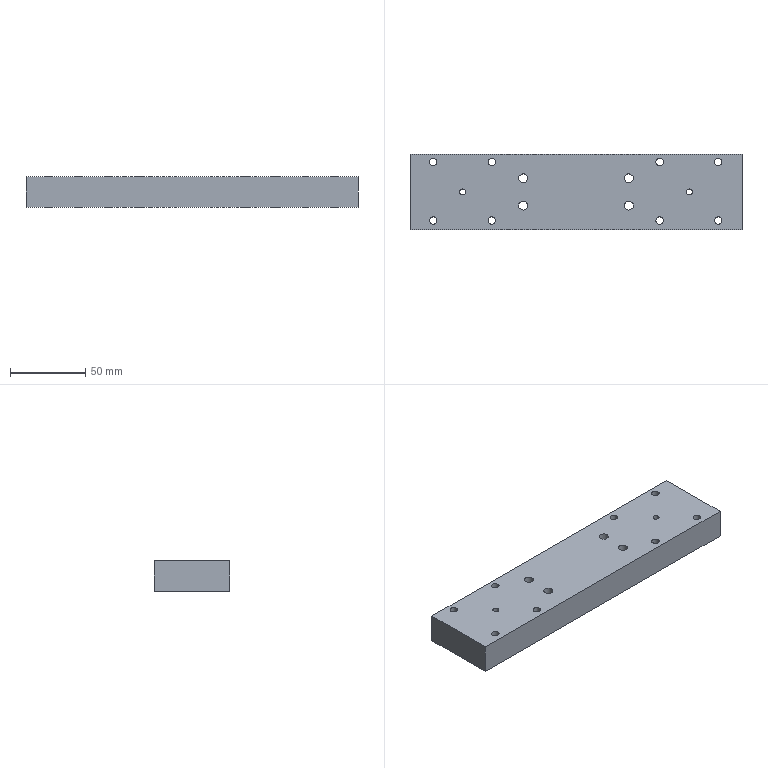NC program | NX | posted with a generic post | part box 220 x 50 x 20 mm
Whole program:
N10 G17 G21 G94 G90
(DRILLING , TOOL : D6A45)
N12 T07 M6
N14 G54
N16 G17 G0 G90 X55.745 Y19.904 S5000 M3
N18 G43 Z30. H7
N20 G94 G81 G98 Z-1. F250. R3.
N22 X94.635
N24 Y-18.987
N26 X75. Y0.
N28 X55.745 Y-18.987
N30 X35. Y-9.
N32 Y9.
N34 X-35.
N36 Y-9.
N38 X-55.365 Y-18.987
N40 X-75. Y0.
N42 X-94.255 Y-18.987
N44 Y19.904
N46 X-55.365
N48 G80
N50 G0 X-55.365 Y19.904 Z30.
N52 M5
(DRILLING_COPY , TOOL : 6.0ZT)
N54 T16 M6
N56 G54
N58 G17 G0 G90 X-35. Y-9. S2000 M3
N60 G43 Z30. H16
N62 G94 G83 G98 Z-23.303 F150. Q2. R3.
N64 Y9.
N66 X35.
N68 Y-9.
N70 G80
N72 G0 X35. Y-9. Z30.
N74 M5
(DRILLING_COPY_COPY , TOOL : 5.0ZT)
N76 T15 M6
N78 G54
N80 G17 G0 G90 X-94.255 Y-18.987 S2000 M3
N82 G43 Z30. H15
N84 G94 G83 G98 Z-23.002 F150. Q2. R3.
N86 Y19.904
N88 X-55.365
N90 Y-18.987
N92 X55.745
N94 X94.635
N96 Y19.904
N98 X55.745
N100 G80
N102 G0 X55.745 Y19.904 Z30.
N104 M5
(DRILLING_COPY_COPY_COPY , TOOL : 3.3ZT)
N106 T14 M6
N108 G54
N110 G17 G0 G90 X75. Y0. S2000 M3
N112 G43 Z30. H14
N114 G94 G83 G98 Z-22.702 F150. Q2. R3.
N116 X-75.
N118 G80
N120 G0 X-75. Y0. Z30.
N122 M5
(PLANAR_MILL_COPY , TOOL : D6A45)
N124 T07 M6
N126 G54
N128 G17 G0 G90 X95.501 Y21.204 S9500 M3
N130 G43 Z30. H7
N132 Z2.
N134 G94 G1 Z-1. F500.
N136 G3 X94.635 Y21.704 R1.
N138 X92.835 Y19.904 R1.8 F1250.
N140 X94.635 Y21.704 R-1.8
N142 X93.769 Y21.204 R1.
N144 G1 Z2.
N146 G0 Z30.
N148 Y-20.287
N150 Z2.
N152 G1 Z-1. F500.
N154 G3 X94.635 Y-20.787 R1.
N156 X96.435 Y-18.987 R1.8 F1250.
N158 X94.635 Y-20.787 R-1.8
N160 X95.501 Y-20.287 R1.
N162 G1 Z2.
N164 G0 Z30.
N166 X74.134 Y-0.8
N168 Z2.
N170 G1 Z-1. F500.
N172 G3 X75. Y-1.3 R1.
N174 X76.3 Y0. R1.3 F1250.
N176 X75. Y-1.3 R-1.3
N178 X75.866 Y-0.8 R1.
N180 G1 Z2.
N182 G0 Z30.
N184 X56.611 Y21.204
N186 Z2.
N188 G1 Z-1. F500.
N190 G3 X55.745 Y21.704 R1.
N192 X53.945 Y19.904 R1.8 F1250.
N194 X55.745 Y21.704 R-1.8
N196 X54.879 Y21.204 R1.
N198 G1 Z2.
N200 G0 Z30.
N202 X35.866 Y10.8
N204 Z2.
N206 G1 Z-1. F500.
N208 G3 X35. Y11.3 R1.
N210 X32.7 Y9. R2.3 F1250.
N212 X35. Y11.3 R-2.3
N214 X34.134 Y10.8 R1.
N216 G1 Z2.
N218 G0 Z30.
N220 X54.879 Y-20.287
N222 Z2.
N224 G1 Z-1. F500.
N226 G3 X55.745 Y-20.787 R1.
N228 X57.545 Y-18.987 R1.8 F1250.
N230 X55.745 Y-20.787 R-1.8
N232 X56.611 Y-20.287 R1.
N234 G1 Z2.
N236 G0 Z30.
N238 X34.134 Y-10.8
N240 Z2.
N242 G1 Z-1. F500.
N244 G3 X35. Y-11.3 R1.
N246 X37.3 Y-9. R2.3 F1250.
N248 X35. Y-11.3 R-2.3
N250 X35.866 Y-10.8 R1.
N252 G1 Z2.
N254 G0 Z30.
N256 X0.866 Y-26.2
N258 Z2.
N260 G1 Z-1. F500.
N262 G3 X0. Y-25.7 R1.
N264 G1 X-110. F1250.
N266 G2 X-110.7 Y-25. R0.7
N268 G1 Y25.
N270 G2 X-110. Y25.7 R0.7
N272 G1 X110.
N274 G2 X110.7 Y25. R0.7
N276 G1 Y-25.
N278 G2 X110. Y-25.7 R0.7
N280 G1 X0.
N282 G3 X-0.866 Y-26.2 R1.
N284 G1 Z2.
N286 G0 Z30.
N288 X-35.866 Y-10.8
N290 Z2.
N292 G1 Z-1. F500.
N294 G3 X-35. Y-11.3 R1.
N296 X-32.7 Y-9. R2.3 F1250.
N298 X-35. Y-11.3 R-2.3
N300 X-34.134 Y-10.8 R1.
N302 G1 Z2.
N304 G0 Z30.
N306 X-56.231 Y-20.287
N308 Z2.
N310 G1 Z-1. F500.
N312 G3 X-55.365 Y-20.787 R1.
N314 X-53.565 Y-18.987 R1.8 F1250.
N316 X-55.365 Y-20.787 R-1.8
N318 X-54.499 Y-20.287 R1.
N320 G1 Z2.
N322 G0 Z30.
N324 X-34.134 Y10.8
N326 Z2.
N328 G1 Z-1. F500.
N330 G3 X-35. Y11.3 R1.
N332 X-37.3 Y9. R2.3 F1250.
N334 X-35. Y11.3 R-2.3
N336 X-35.866 Y10.8 R1.
N338 G1 Z2.
N340 G0 Z30.
N342 X-54.499 Y21.204
N344 Z2.
N346 G1 Z-1. F500.
N348 G3 X-55.365 Y21.704 R1.
N350 X-57.165 Y19.904 R1.8 F1250.
N352 X-55.365 Y21.704 R-1.8
N354 X-56.231 Y21.204 R1.
N356 G1 Z2.
N358 G0 Z30.
N360 X-93.389
N362 Z2.
N364 G1 Z-1. F500.
N366 G3 X-94.255 Y21.704 R1.
N368 X-96.055 Y19.904 R1.8 F1250.
N370 X-94.255 Y21.704 R-1.8
N372 X-95.121 Y21.204 R1.
N374 G1 Z2.
N376 G0 Z30.
N378 X-74.134 Y0.8
N380 Z2.
N382 G1 Z-1. F500.
N384 G3 X-75. Y1.3 R1.
N386 X-76.3 Y0. R1.3 F1250.
N388 X-75. Y1.3 R-1.3
N390 X-75.866 Y0.8 R1.
N392 G1 Z2.
N394 G0 Z30.
N396 X-95.121 Y-20.287
N398 Z2.
N400 G1 Z-1. F500.
N402 G3 X-94.255 Y-20.787 R1.
N404 X-92.455 Y-18.987 R1.8 F1250.
N406 X-94.255 Y-20.787 R-1.8
N408 X-93.389 Y-20.287 R1.
N410 G1 Z2.
N412 G0 Z30.
N414 M5
N416 M2